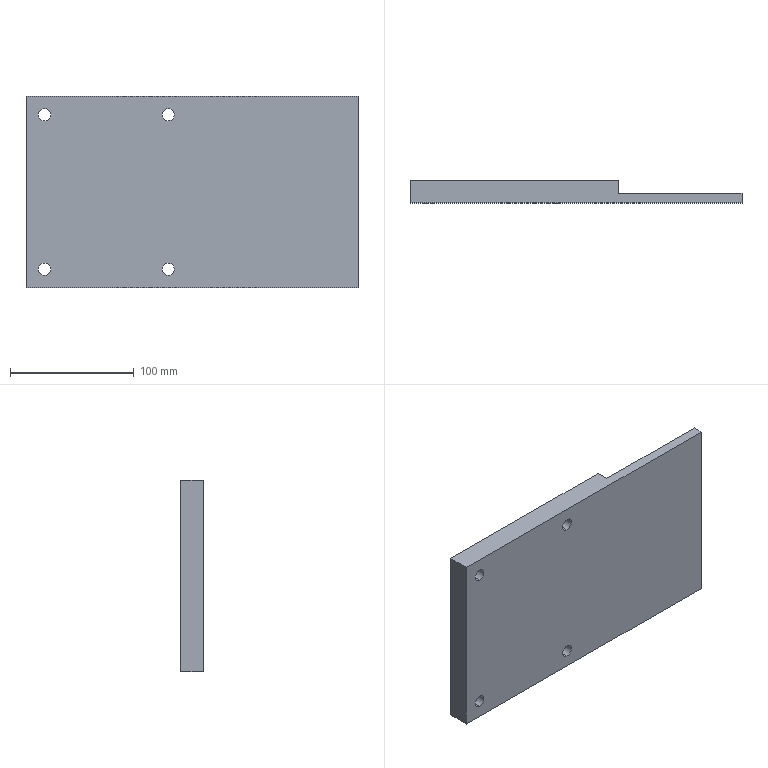Part | SolidWorks | features ICE 2, Extrusion 1 | 1 solid | 16 faces | box 268.5 x 18 x 155 mm | volume 588460 mm3 | cylinder 8 | plane 8 | commonest cylinder face diameters 10 x8
STEP:
#1=CARTESIAN_POINT('',(-119.25,0.,57.5));
#2=VERTEX_POINT('',#1);
#3=CARTESIAN_POINT('',(-119.25,0.,67.5));
#4=VERTEX_POINT('',#3);
#5=CARTESIAN_POINT('',(-119.25,0.,62.5));
#6=DIRECTION('',(0.,1.,0.));
#7=DIRECTION('',(0.,0.,-1.));
#8=AXIS2_PLACEMENT_3D('',#5,#6,#7);
#9=CIRCLE('',#8,5.);
#10=EDGE_CURVE('',#2,#4,#9,.T.);
#11=ORIENTED_EDGE('',*,*,#10,.F.);
#12=CARTESIAN_POINT('',(-119.25,18.,57.5));
#13=VERTEX_POINT('',#12);
#14=CARTESIAN_POINT('',(-119.25,0.,57.5));
#15=DIRECTION('',(0.,1.,0.));
#16=VECTOR('',#15,1000.);
#17=LINE('',#14,#16);
#18=EDGE_CURVE('',#2,#13,#17,.T.);
#19=ORIENTED_EDGE('',*,*,#18,.T.);
#20=CARTESIAN_POINT('',(-119.25,18.,67.5));
#21=VERTEX_POINT('',#20);
#22=CARTESIAN_POINT('',(-119.25,18.,62.5));
#23=DIRECTION('',(0.,1.,0.));
#24=DIRECTION('',(0.,0.,-1.));
#25=AXIS2_PLACEMENT_3D('',#22,#23,#24);
#26=CIRCLE('',#25,5.);
#27=EDGE_CURVE('',#13,#21,#26,.T.);
#28=ORIENTED_EDGE('',*,*,#27,.T.);
#29=CARTESIAN_POINT('',(-119.25,0.,67.5));
#30=DIRECTION('',(0.,1.,0.));
#31=VECTOR('',#30,1000.);
#32=LINE('',#29,#31);
#33=EDGE_CURVE('',#4,#21,#32,.T.);
#34=ORIENTED_EDGE('',*,*,#33,.F.);
#35=EDGE_LOOP('',(#11,#19,#28,#34));
#36=FACE_OUTER_BOUND('',#35,.T.);
#37=CARTESIAN_POINT('',(-119.25,0.,62.5));
#38=DIRECTION('',(0.,1.,0.));
#39=DIRECTION('',(0.,0.,1.));
#40=AXIS2_PLACEMENT_3D('',#37,#38,#39);
#41=CYLINDRICAL_SURFACE('',#40,5.);
#42=ADVANCED_FACE('',(#36),#41,.F.);
#43=CARTESIAN_POINT('',(-19.25,0.,57.5));
#44=VERTEX_POINT('',#43);
#45=CARTESIAN_POINT('',(-19.25,0.,67.5));
#46=VERTEX_POINT('',#45);
#47=CARTESIAN_POINT('',(-19.25,0.,62.5));
#48=DIRECTION('',(0.,1.,0.));
#49=DIRECTION('',(0.,0.,-1.));
#50=AXIS2_PLACEMENT_3D('',#47,#48,#49);
#51=CIRCLE('',#50,5.);
#52=EDGE_CURVE('',#44,#46,#51,.T.);
#53=ORIENTED_EDGE('',*,*,#52,.F.);
#54=CARTESIAN_POINT('',(-19.25,18.,57.5));
#55=VERTEX_POINT('',#54);
#56=CARTESIAN_POINT('',(-19.25,0.,57.5));
#57=DIRECTION('',(0.,1.,0.));
#58=VECTOR('',#57,1000.);
#59=LINE('',#56,#58);
#60=EDGE_CURVE('',#44,#55,#59,.T.);
#61=ORIENTED_EDGE('',*,*,#60,.T.);
#62=CARTESIAN_POINT('',(-19.25,18.,67.5));
#63=VERTEX_POINT('',#62);
#64=CARTESIAN_POINT('',(-19.25,18.,62.5));
#65=DIRECTION('',(0.,1.,0.));
#66=DIRECTION('',(0.,0.,-1.));
#67=AXIS2_PLACEMENT_3D('',#64,#65,#66);
#68=CIRCLE('',#67,5.);
#69=EDGE_CURVE('',#55,#63,#68,.T.);
#70=ORIENTED_EDGE('',*,*,#69,.T.);
#71=CARTESIAN_POINT('',(-19.25,0.,67.5));
#72=DIRECTION('',(0.,1.,0.));
#73=VECTOR('',#72,1000.);
#74=LINE('',#71,#73);
#75=EDGE_CURVE('',#46,#63,#74,.T.);
#76=ORIENTED_EDGE('',*,*,#75,.F.);
#77=EDGE_LOOP('',(#53,#61,#70,#76));
#78=FACE_OUTER_BOUND('',#77,.T.);
#79=CARTESIAN_POINT('',(-19.25,0.,62.5));
#80=DIRECTION('',(0.,1.,0.));
#81=DIRECTION('',(0.,0.,1.));
#82=AXIS2_PLACEMENT_3D('',#79,#80,#81);
#83=CYLINDRICAL_SURFACE('',#82,5.);
#84=ADVANCED_FACE('',(#78),#83,.F.);
#85=CARTESIAN_POINT('',(-19.25,0.,-67.5));
#86=VERTEX_POINT('',#85);
#87=CARTESIAN_POINT('',(-19.25,0.,-57.5));
#88=VERTEX_POINT('',#87);
#89=CARTESIAN_POINT('',(-19.25,0.,-62.5));
#90=DIRECTION('',(0.,1.,0.));
#91=DIRECTION('',(0.,0.,1.));
#92=AXIS2_PLACEMENT_3D('',#89,#90,#91);
#93=CIRCLE('',#92,5.);
#94=EDGE_CURVE('',#86,#88,#93,.T.);
#95=ORIENTED_EDGE('',*,*,#94,.F.);
#96=CARTESIAN_POINT('',(-19.25,18.,-67.5));
#97=VERTEX_POINT('',#96);
#98=CARTESIAN_POINT('',(-19.25,0.,-67.5));
#99=DIRECTION('',(0.,1.,0.));
#100=VECTOR('',#99,1000.);
#101=LINE('',#98,#100);
#102=EDGE_CURVE('',#86,#97,#101,.T.);
#103=ORIENTED_EDGE('',*,*,#102,.T.);
#104=CARTESIAN_POINT('',(-19.25,18.,-57.5));
#105=VERTEX_POINT('',#104);
#106=CARTESIAN_POINT('',(-19.25,18.,-62.5));
#107=DIRECTION('',(0.,1.,0.));
#108=DIRECTION('',(0.,0.,1.));
#109=AXIS2_PLACEMENT_3D('',#106,#107,#108);
#110=CIRCLE('',#109,5.);
#111=EDGE_CURVE('',#97,#105,#110,.T.);
#112=ORIENTED_EDGE('',*,*,#111,.T.);
#113=CARTESIAN_POINT('',(-19.25,0.,-57.5));
#114=DIRECTION('',(0.,1.,0.));
#115=VECTOR('',#114,1000.);
#116=LINE('',#113,#115);
#117=EDGE_CURVE('',#88,#105,#116,.T.);
#118=ORIENTED_EDGE('',*,*,#117,.F.);
#119=EDGE_LOOP('',(#95,#103,#112,#118));
#120=FACE_OUTER_BOUND('',#119,.T.);
#121=CARTESIAN_POINT('',(-19.25,0.,-62.5));
#122=DIRECTION('',(0.,1.,0.));
#123=DIRECTION('',(0.,0.,1.));
#124=AXIS2_PLACEMENT_3D('',#121,#122,#123);
#125=CYLINDRICAL_SURFACE('',#124,5.);
#126=ADVANCED_FACE('',(#120),#125,.F.);
#127=CARTESIAN_POINT('',(-119.25,0.,-67.5));
#128=VERTEX_POINT('',#127);
#129=CARTESIAN_POINT('',(-119.25,0.,-57.5));
#130=VERTEX_POINT('',#129);
#131=CARTESIAN_POINT('',(-119.25,0.,-62.5));
#132=DIRECTION('',(0.,1.,0.));
#133=DIRECTION('',(0.,0.,1.));
#134=AXIS2_PLACEMENT_3D('',#131,#132,#133);
#135=CIRCLE('',#134,5.);
#136=EDGE_CURVE('',#128,#130,#135,.T.);
#137=ORIENTED_EDGE('',*,*,#136,.F.);
#138=CARTESIAN_POINT('',(-119.25,18.,-67.5));
#139=VERTEX_POINT('',#138);
#140=CARTESIAN_POINT('',(-119.25,0.,-67.5));
#141=DIRECTION('',(0.,1.,0.));
#142=VECTOR('',#141,1000.);
#143=LINE('',#140,#142);
#144=EDGE_CURVE('',#128,#139,#143,.T.);
#145=ORIENTED_EDGE('',*,*,#144,.T.);
#146=CARTESIAN_POINT('',(-119.25,18.,-57.5));
#147=VERTEX_POINT('',#146);
#148=CARTESIAN_POINT('',(-119.25,18.,-62.5));
#149=DIRECTION('',(0.,1.,0.));
#150=DIRECTION('',(0.,0.,1.));
#151=AXIS2_PLACEMENT_3D('',#148,#149,#150);
#152=CIRCLE('',#151,5.);
#153=EDGE_CURVE('',#139,#147,#152,.T.);
#154=ORIENTED_EDGE('',*,*,#153,.T.);
#155=CARTESIAN_POINT('',(-119.25,0.,-57.5));
#156=DIRECTION('',(0.,1.,0.));
#157=VECTOR('',#156,1000.);
#158=LINE('',#155,#157);
#159=EDGE_CURVE('',#130,#147,#158,.T.);
#160=ORIENTED_EDGE('',*,*,#159,.F.);
#161=EDGE_LOOP('',(#137,#145,#154,#160));
#162=FACE_OUTER_BOUND('',#161,.T.);
#163=CARTESIAN_POINT('',(-119.25,0.,-62.5));
#164=DIRECTION('',(0.,1.,0.));
#165=DIRECTION('',(0.,0.,1.));
#166=AXIS2_PLACEMENT_3D('',#163,#164,#165);
#167=CYLINDRICAL_SURFACE('',#166,5.);
#168=ADVANCED_FACE('',(#162),#167,.F.);
#169=CARTESIAN_POINT('',(134.25,8.,-77.5));
#170=VERTEX_POINT('',#169);
#171=CARTESIAN_POINT('',(134.25,0.,-77.5));
#172=VERTEX_POINT('',#171);
#173=CARTESIAN_POINT('',(134.25,18.,-77.5));
#174=DIRECTION('',(0.,-1.,0.));
#175=VECTOR('',#174,1000.);
#176=LINE('',#173,#175);
#177=EDGE_CURVE('',#170,#172,#176,.T.);
#178=ORIENTED_EDGE('',*,*,#177,.F.);
#179=CARTESIAN_POINT('',(134.25,8.,77.5));
#180=VERTEX_POINT('',#179);
#181=CARTESIAN_POINT('',(134.25,8.,-77.5));
#182=DIRECTION('',(0.,0.,-1.));
#183=VECTOR('',#182,1000.);
#184=LINE('',#181,#183);
#185=EDGE_CURVE('',#180,#170,#184,.T.);
#186=ORIENTED_EDGE('',*,*,#185,.F.);
#187=CARTESIAN_POINT('',(134.25,0.,77.5));
#188=VERTEX_POINT('',#187);
#189=CARTESIAN_POINT('',(134.25,18.,77.5));
#190=DIRECTION('',(0.,-1.,0.));
#191=VECTOR('',#190,1000.);
#192=LINE('',#189,#191);
#193=EDGE_CURVE('',#180,#188,#192,.T.);
#194=ORIENTED_EDGE('',*,*,#193,.T.);
#195=CARTESIAN_POINT('',(134.25,0.,77.5));
#196=DIRECTION('',(0.,0.,-1.));
#197=VECTOR('',#196,1000.);
#198=LINE('',#195,#197);
#199=EDGE_CURVE('',#188,#172,#198,.T.);
#200=ORIENTED_EDGE('',*,*,#199,.T.);
#201=EDGE_LOOP('',(#178,#186,#194,#200));
#202=FACE_OUTER_BOUND('',#201,.T.);
#203=CARTESIAN_POINT('',(134.25,18.,77.5));
#204=DIRECTION('',(-1.,0.,0.));
#205=DIRECTION('',(0.,0.,1.));
#206=AXIS2_PLACEMENT_3D('',#203,#204,#205);
#207=PLANE('',#206);
#208=ADVANCED_FACE('',(#202),#207,.F.);
#209=CARTESIAN_POINT('',(34.25,18.,-77.5));
#210=VERTEX_POINT('',#209);
#211=CARTESIAN_POINT('',(-134.25,18.,-77.5));
#212=VERTEX_POINT('',#211);
#213=CARTESIAN_POINT('',(-134.25,18.,-77.5));
#214=DIRECTION('',(-1.,0.,0.));
#215=VECTOR('',#214,1000.);
#216=LINE('',#213,#215);
#217=EDGE_CURVE('',#210,#212,#216,.T.);
#218=ORIENTED_EDGE('',*,*,#217,.F.);
#219=CARTESIAN_POINT('',(34.25,8.,-77.5));
#220=VERTEX_POINT('',#219);
#221=CARTESIAN_POINT('',(34.25,8.,-77.5));
#222=DIRECTION('',(0.,1.,0.));
#223=VECTOR('',#222,1000.);
#224=LINE('',#221,#223);
#225=EDGE_CURVE('',#220,#210,#224,.T.);
#226=ORIENTED_EDGE('',*,*,#225,.F.);
#227=CARTESIAN_POINT('',(134.25,8.,-77.5));
#228=DIRECTION('',(-1.,0.,0.));
#229=VECTOR('',#228,1000.);
#230=LINE('',#227,#229);
#231=EDGE_CURVE('',#170,#220,#230,.T.);
#232=ORIENTED_EDGE('',*,*,#231,.F.);
#233=ORIENTED_EDGE('',*,*,#177,.T.);
#234=CARTESIAN_POINT('',(-134.25,0.,-77.5));
#235=VERTEX_POINT('',#234);
#236=CARTESIAN_POINT('',(-134.25,0.,-77.5));
#237=DIRECTION('',(-1.,0.,0.));
#238=VECTOR('',#237,1000.);
#239=LINE('',#236,#238);
#240=EDGE_CURVE('',#172,#235,#239,.T.);
#241=ORIENTED_EDGE('',*,*,#240,.T.);
#242=CARTESIAN_POINT('',(-134.25,18.,-77.5));
#243=DIRECTION('',(0.,-1.,0.));
#244=VECTOR('',#243,1000.);
#245=LINE('',#242,#244);
#246=EDGE_CURVE('',#212,#235,#245,.T.);
#247=ORIENTED_EDGE('',*,*,#246,.F.);
#248=EDGE_LOOP('',(#218,#226,#232,#233,#241,#247));
#249=FACE_OUTER_BOUND('',#248,.T.);
#250=CARTESIAN_POINT('',(-134.25,18.,-77.5));
#251=DIRECTION('',(0.,0.,1.));
#252=DIRECTION('',(1.,0.,0.));
#253=AXIS2_PLACEMENT_3D('',#250,#251,#252);
#254=PLANE('',#253);
#255=ADVANCED_FACE('',(#249),#254,.F.);
#256=CARTESIAN_POINT('',(-134.25,0.,77.5));
#257=VERTEX_POINT('',#256);
#258=CARTESIAN_POINT('',(-134.25,0.,77.5));
#259=DIRECTION('',(0.,0.,1.));
#260=VECTOR('',#259,1000.);
#261=LINE('',#258,#260);
#262=EDGE_CURVE('',#235,#257,#261,.T.);
#263=ORIENTED_EDGE('',*,*,#262,.T.);
#264=CARTESIAN_POINT('',(-134.25,18.,77.5));
#265=VERTEX_POINT('',#264);
#266=CARTESIAN_POINT('',(-134.25,18.,77.5));
#267=DIRECTION('',(0.,-1.,0.));
#268=VECTOR('',#267,1000.);
#269=LINE('',#266,#268);
#270=EDGE_CURVE('',#265,#257,#269,.T.);
#271=ORIENTED_EDGE('',*,*,#270,.F.);
#272=CARTESIAN_POINT('',(-134.25,18.,77.5));
#273=DIRECTION('',(0.,0.,1.));
#274=VECTOR('',#273,1000.);
#275=LINE('',#272,#274);
#276=EDGE_CURVE('',#212,#265,#275,.T.);
#277=ORIENTED_EDGE('',*,*,#276,.F.);
#278=ORIENTED_EDGE('',*,*,#246,.T.);
#279=EDGE_LOOP('',(#263,#271,#277,#278));
#280=FACE_OUTER_BOUND('',#279,.T.);
#281=CARTESIAN_POINT('',(-134.25,18.,77.5));
#282=DIRECTION('',(1.,0.,0.));
#283=DIRECTION('',(0.,0.,-1.));
#284=AXIS2_PLACEMENT_3D('',#281,#282,#283);
#285=PLANE('',#284);
#286=ADVANCED_FACE('',(#280),#285,.F.);
#287=CARTESIAN_POINT('',(34.25,8.,77.5));
#288=VERTEX_POINT('',#287);
#289=CARTESIAN_POINT('',(134.25,8.,77.5));
#290=DIRECTION('',(1.,0.,0.));
#291=VECTOR('',#290,1000.);
#292=LINE('',#289,#291);
#293=EDGE_CURVE('',#288,#180,#292,.T.);
#294=ORIENTED_EDGE('',*,*,#293,.F.);
#295=CARTESIAN_POINT('',(34.25,18.,77.5));
#296=VERTEX_POINT('',#295);
#297=CARTESIAN_POINT('',(34.25,8.,77.5));
#298=DIRECTION('',(0.,1.,0.));
#299=VECTOR('',#298,1000.);
#300=LINE('',#297,#299);
#301=EDGE_CURVE('',#288,#296,#300,.T.);
#302=ORIENTED_EDGE('',*,*,#301,.T.);
#303=CARTESIAN_POINT('',(-134.25,18.,77.5));
#304=DIRECTION('',(1.,0.,0.));
#305=VECTOR('',#304,1000.);
#306=LINE('',#303,#305);
#307=EDGE_CURVE('',#265,#296,#306,.T.);
#308=ORIENTED_EDGE('',*,*,#307,.F.);
#309=ORIENTED_EDGE('',*,*,#270,.T.);
#310=CARTESIAN_POINT('',(-134.25,0.,77.5));
#311=DIRECTION('',(1.,0.,0.));
#312=VECTOR('',#311,1000.);
#313=LINE('',#310,#312);
#314=EDGE_CURVE('',#257,#188,#313,.T.);
#315=ORIENTED_EDGE('',*,*,#314,.T.);
#316=ORIENTED_EDGE('',*,*,#193,.F.);
#317=EDGE_LOOP('',(#294,#302,#308,#309,#315,#316));
#318=FACE_OUTER_BOUND('',#317,.T.);
#319=CARTESIAN_POINT('',(-134.25,18.,77.5));
#320=DIRECTION('',(0.,0.,-1.));
#321=DIRECTION('',(-1.,0.,0.));
#322=AXIS2_PLACEMENT_3D('',#319,#320,#321);
#323=PLANE('',#322);
#324=ADVANCED_FACE('',(#318),#323,.F.);
#325=CARTESIAN_POINT('',(-119.25,18.,62.5));
#326=DIRECTION('',(0.,1.,0.));
#327=DIRECTION('',(0.,0.,-1.));
#328=AXIS2_PLACEMENT_3D('',#325,#326,#327);
#329=CIRCLE('',#328,5.);
#330=EDGE_CURVE('',#21,#13,#329,.T.);
#331=ORIENTED_EDGE('',*,*,#330,.F.);
#332=ORIENTED_EDGE('',*,*,#27,.F.);
#333=EDGE_LOOP('',(#331,#332));
#334=FACE_BOUND('',#333,.T.);
#335=CARTESIAN_POINT('',(-19.25,18.,62.5));
#336=DIRECTION('',(0.,1.,0.));
#337=DIRECTION('',(0.,0.,-1.));
#338=AXIS2_PLACEMENT_3D('',#335,#336,#337);
#339=CIRCLE('',#338,5.);
#340=EDGE_CURVE('',#63,#55,#339,.T.);
#341=ORIENTED_EDGE('',*,*,#340,.F.);
#342=ORIENTED_EDGE('',*,*,#69,.F.);
#343=EDGE_LOOP('',(#341,#342));
#344=FACE_BOUND('',#343,.T.);
#345=CARTESIAN_POINT('',(-19.25,18.,-62.5));
#346=DIRECTION('',(0.,1.,0.));
#347=DIRECTION('',(0.,0.,1.));
#348=AXIS2_PLACEMENT_3D('',#345,#346,#347);
#349=CIRCLE('',#348,5.);
#350=EDGE_CURVE('',#105,#97,#349,.T.);
#351=ORIENTED_EDGE('',*,*,#350,.F.);
#352=ORIENTED_EDGE('',*,*,#111,.F.);
#353=EDGE_LOOP('',(#351,#352));
#354=FACE_BOUND('',#353,.T.);
#355=CARTESIAN_POINT('',(-119.25,18.,-62.5));
#356=DIRECTION('',(0.,1.,0.));
#357=DIRECTION('',(0.,0.,1.));
#358=AXIS2_PLACEMENT_3D('',#355,#356,#357);
#359=CIRCLE('',#358,5.);
#360=EDGE_CURVE('',#147,#139,#359,.T.);
#361=ORIENTED_EDGE('',*,*,#360,.F.);
#362=ORIENTED_EDGE('',*,*,#153,.F.);
#363=EDGE_LOOP('',(#361,#362));
#364=FACE_BOUND('',#363,.T.);
#365=ORIENTED_EDGE('',*,*,#307,.T.);
#366=CARTESIAN_POINT('',(34.25,18.,-77.5));
#367=DIRECTION('',(0.,0.,1.));
#368=VECTOR('',#367,1000.);
#369=LINE('',#366,#368);
#370=EDGE_CURVE('',#210,#296,#369,.T.);
#371=ORIENTED_EDGE('',*,*,#370,.F.);
#372=ORIENTED_EDGE('',*,*,#217,.T.);
#373=ORIENTED_EDGE('',*,*,#276,.T.);
#374=EDGE_LOOP('',(#365,#371,#372,#373));
#375=FACE_OUTER_BOUND('',#374,.T.);
#376=CARTESIAN_POINT('',(0.,18.,0.));
#377=DIRECTION('',(0.,-1.,0.));
#378=DIRECTION('',(0.,0.,-1.));
#379=AXIS2_PLACEMENT_3D('',#376,#377,#378);
#380=PLANE('',#379);
#381=ADVANCED_FACE('',(#334,#344,#354,#364,#375),#380,.F.);
#382=CARTESIAN_POINT('',(-119.25,0.,62.5));
#383=DIRECTION('',(0.,1.,0.));
#384=DIRECTION('',(0.,0.,-1.));
#385=AXIS2_PLACEMENT_3D('',#382,#383,#384);
#386=CIRCLE('',#385,5.);
#387=EDGE_CURVE('',#4,#2,#386,.T.);
#388=ORIENTED_EDGE('',*,*,#387,.T.);
#389=ORIENTED_EDGE('',*,*,#10,.T.);
#390=EDGE_LOOP('',(#388,#389));
#391=FACE_BOUND('',#390,.T.);
#392=CARTESIAN_POINT('',(-19.25,0.,62.5));
#393=DIRECTION('',(0.,1.,0.));
#394=DIRECTION('',(0.,0.,-1.));
#395=AXIS2_PLACEMENT_3D('',#392,#393,#394);
#396=CIRCLE('',#395,5.);
#397=EDGE_CURVE('',#46,#44,#396,.T.);
#398=ORIENTED_EDGE('',*,*,#397,.T.);
#399=ORIENTED_EDGE('',*,*,#52,.T.);
#400=EDGE_LOOP('',(#398,#399));
#401=FACE_BOUND('',#400,.T.);
#402=CARTESIAN_POINT('',(-19.25,0.,-62.5));
#403=DIRECTION('',(0.,1.,0.));
#404=DIRECTION('',(0.,0.,1.));
#405=AXIS2_PLACEMENT_3D('',#402,#403,#404);
#406=CIRCLE('',#405,5.);
#407=EDGE_CURVE('',#88,#86,#406,.T.);
#408=ORIENTED_EDGE('',*,*,#407,.T.);
#409=ORIENTED_EDGE('',*,*,#94,.T.);
#410=EDGE_LOOP('',(#408,#409));
#411=FACE_BOUND('',#410,.T.);
#412=CARTESIAN_POINT('',(-119.25,0.,-62.5));
#413=DIRECTION('',(0.,1.,0.));
#414=DIRECTION('',(0.,0.,1.));
#415=AXIS2_PLACEMENT_3D('',#412,#413,#414);
#416=CIRCLE('',#415,5.);
#417=EDGE_CURVE('',#130,#128,#416,.T.);
#418=ORIENTED_EDGE('',*,*,#417,.T.);
#419=ORIENTED_EDGE('',*,*,#136,.T.);
#420=EDGE_LOOP('',(#418,#419));
#421=FACE_BOUND('',#420,.T.);
#422=ORIENTED_EDGE('',*,*,#199,.F.);
#423=ORIENTED_EDGE('',*,*,#314,.F.);
#424=ORIENTED_EDGE('',*,*,#262,.F.);
#425=ORIENTED_EDGE('',*,*,#240,.F.);
#426=EDGE_LOOP('',(#422,#423,#424,#425));
#427=FACE_OUTER_BOUND('',#426,.T.);
#428=CARTESIAN_POINT('',(0.,0.,0.));
#429=DIRECTION('',(0.,-1.,0.));
#430=DIRECTION('',(0.,0.,-1.));
#431=AXIS2_PLACEMENT_3D('',#428,#429,#430);
#432=PLANE('',#431);
#433=ADVANCED_FACE('',(#391,#401,#411,#421,#427),#432,.T.);
#434=ORIENTED_EDGE('',*,*,#144,.F.);
#435=ORIENTED_EDGE('',*,*,#417,.F.);
#436=ORIENTED_EDGE('',*,*,#159,.T.);
#437=ORIENTED_EDGE('',*,*,#360,.T.);
#438=EDGE_LOOP('',(#434,#435,#436,#437));
#439=FACE_OUTER_BOUND('',#438,.T.);
#440=CARTESIAN_POINT('',(-119.25,0.,-62.5));
#441=DIRECTION('',(0.,1.,0.));
#442=DIRECTION('',(0.,0.,1.));
#443=AXIS2_PLACEMENT_3D('',#440,#441,#442);
#444=CYLINDRICAL_SURFACE('',#443,5.);
#445=ADVANCED_FACE('',(#439),#444,.F.);
#446=ORIENTED_EDGE('',*,*,#102,.F.);
#447=ORIENTED_EDGE('',*,*,#407,.F.);
#448=ORIENTED_EDGE('',*,*,#117,.T.);
#449=ORIENTED_EDGE('',*,*,#350,.T.);
#450=EDGE_LOOP('',(#446,#447,#448,#449));
#451=FACE_OUTER_BOUND('',#450,.T.);
#452=CARTESIAN_POINT('',(-19.25,0.,-62.5));
#453=DIRECTION('',(0.,1.,0.));
#454=DIRECTION('',(0.,0.,1.));
#455=AXIS2_PLACEMENT_3D('',#452,#453,#454);
#456=CYLINDRICAL_SURFACE('',#455,5.);
#457=ADVANCED_FACE('',(#451),#456,.F.);
#458=ORIENTED_EDGE('',*,*,#60,.F.);
#459=ORIENTED_EDGE('',*,*,#397,.F.);
#460=ORIENTED_EDGE('',*,*,#75,.T.);
#461=ORIENTED_EDGE('',*,*,#340,.T.);
#462=EDGE_LOOP('',(#458,#459,#460,#461));
#463=FACE_OUTER_BOUND('',#462,.T.);
#464=CARTESIAN_POINT('',(-19.25,0.,62.5));
#465=DIRECTION('',(0.,1.,0.));
#466=DIRECTION('',(0.,0.,1.));
#467=AXIS2_PLACEMENT_3D('',#464,#465,#466);
#468=CYLINDRICAL_SURFACE('',#467,5.);
#469=ADVANCED_FACE('',(#463),#468,.F.);
#470=ORIENTED_EDGE('',*,*,#18,.F.);
#471=ORIENTED_EDGE('',*,*,#387,.F.);
#472=ORIENTED_EDGE('',*,*,#33,.T.);
#473=ORIENTED_EDGE('',*,*,#330,.T.);
#474=EDGE_LOOP('',(#470,#471,#472,#473));
#475=FACE_OUTER_BOUND('',#474,.T.);
#476=CARTESIAN_POINT('',(-119.25,0.,62.5));
#477=DIRECTION('',(0.,1.,0.));
#478=DIRECTION('',(0.,0.,1.));
#479=AXIS2_PLACEMENT_3D('',#476,#477,#478);
#480=CYLINDRICAL_SURFACE('',#479,5.);
#481=ADVANCED_FACE('',(#475),#480,.F.);
#482=ORIENTED_EDGE('',*,*,#370,.T.);
#483=ORIENTED_EDGE('',*,*,#301,.F.);
#484=CARTESIAN_POINT('',(34.25,8.,-77.5));
#485=DIRECTION('',(0.,0.,1.));
#486=VECTOR('',#485,1000.);
#487=LINE('',#484,#486);
#488=EDGE_CURVE('',#220,#288,#487,.T.);
#489=ORIENTED_EDGE('',*,*,#488,.F.);
#490=ORIENTED_EDGE('',*,*,#225,.T.);
#491=EDGE_LOOP('',(#482,#483,#489,#490));
#492=FACE_OUTER_BOUND('',#491,.T.);
#493=CARTESIAN_POINT('',(34.25,8.,-77.5));
#494=DIRECTION('',(-1.,0.,0.));
#495=DIRECTION('',(0.,0.,1.));
#496=AXIS2_PLACEMENT_3D('',#493,#494,#495);
#497=PLANE('',#496);
#498=ADVANCED_FACE('',(#492),#497,.F.);
#499=ORIENTED_EDGE('',*,*,#185,.T.);
#500=ORIENTED_EDGE('',*,*,#231,.T.);
#501=ORIENTED_EDGE('',*,*,#488,.T.);
#502=ORIENTED_EDGE('',*,*,#293,.T.);
#503=EDGE_LOOP('',(#499,#500,#501,#502));
#504=FACE_OUTER_BOUND('',#503,.T.);
#505=CARTESIAN_POINT('',(0.,8.,0.));
#506=DIRECTION('',(0.,-1.,0.));
#507=DIRECTION('',(0.,0.,-1.));
#508=AXIS2_PLACEMENT_3D('',#505,#506,#507);
#509=PLANE('',#508);
#510=ADVANCED_FACE('',(#504),#509,.F.);
#511=CLOSED_SHELL('',(#42,#84,#126,#168,#208,#255,#286,#324,#381,#433,#445,#457,#469,#481,#498,#510));
#512=MANIFOLD_SOLID_BREP('',#511);
#513=CARTESIAN_POINT('',(0.,0.,0.));
#514=DIRECTION('',(0.,0.,1.));
#515=DIRECTION('',(1.,0.,0.));
#516=AXIS2_PLACEMENT_3D('',#513,#514,#515);
#517=(LENGTH_UNIT()NAMED_UNIT(*)SI_UNIT(.MILLI.,.METRE.));
#518=UNCERTAINTY_MEASURE_WITH_UNIT(LENGTH_MEASURE(0.00001),#517,'','');
#519=(NAMED_UNIT(*)PLANE_ANGLE_UNIT()SI_UNIT($,.RADIAN.));
#520=(NAMED_UNIT(*)SI_UNIT($,.STERADIAN.)SOLID_ANGLE_UNIT());
#521=(GEOMETRIC_REPRESENTATION_CONTEXT(3)GLOBAL_UNCERTAINTY_ASSIGNED_CONTEXT((#518))GLOBAL_UNIT_ASSIGNED_CONTEXT((#517,#519,#520))REPRESENTATION_CONTEXT('',''));
#522=ADVANCED_BREP_SHAPE_REPRESENTATION('',(#512,#516),#521);